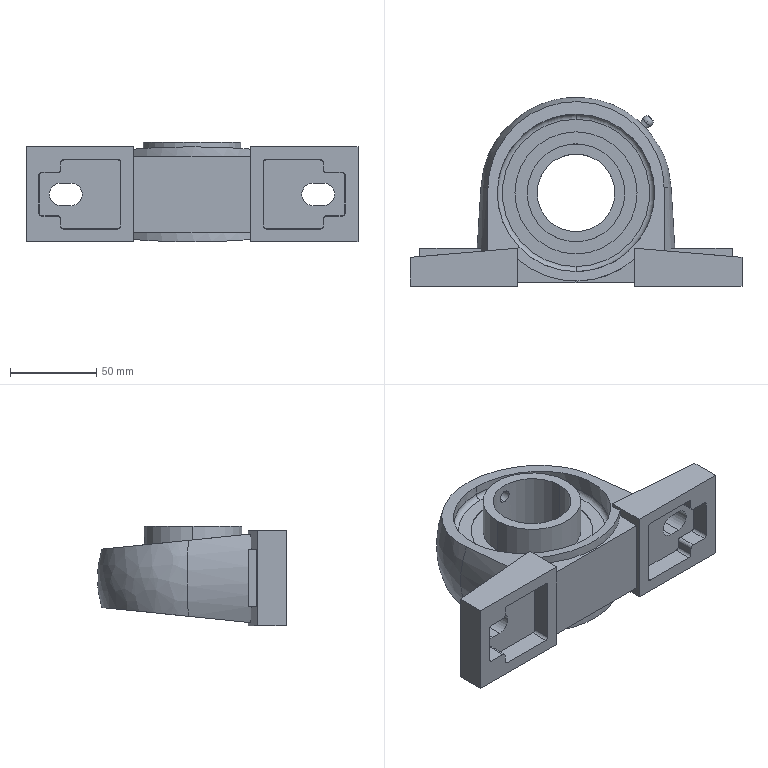Part | SolidWorks | features Revolution 5, Boss 3, Cut 3, RevCut 2, CirPattern 1, Extrusion 1, SweepCut 1 | 1 solid | 121 faces | box 192 x 109.26 x 57.7 mm | volume 325888 mm3 | plane 58 | cylinder 28 | cone 16 | sphere 8 | torus 8 | spline 3 | commonest cylinder face diameters 56.6 x6 70.64 x6 91.076 x6 13 x4 7.134 x2 45 x2